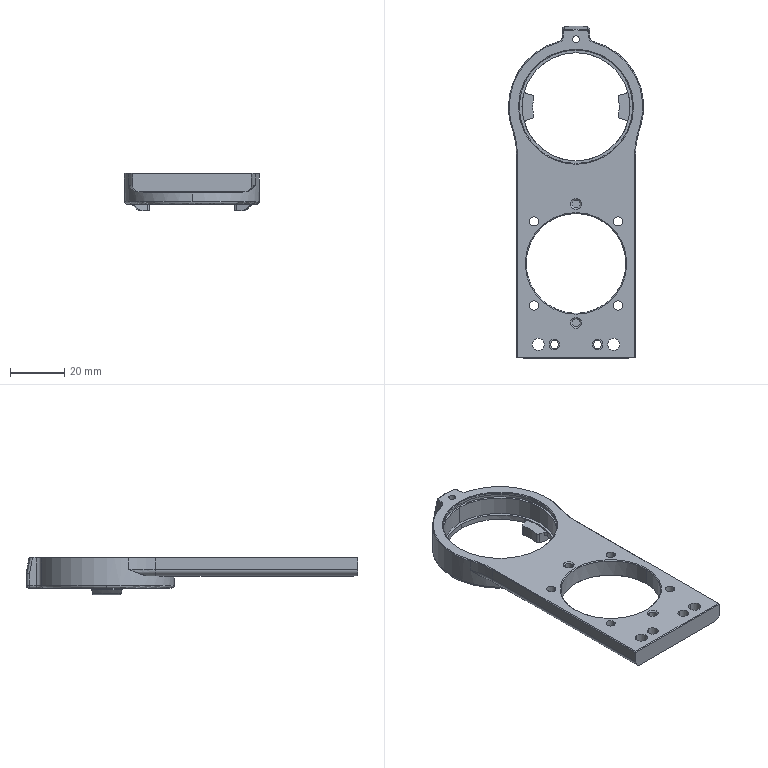NC program | NX | posted with a generic post | part box 50 x 122.9 x 14 mm
Lines 1 to 868 of 10876:
N10 G17 G21 G94 G90
(FLOOR_WALL_COPY , TOOL : D80)
N12 T19 M6
N14 G54
N16 G17 G0 G90 X-45. Y0. S5000 M3
N18 G43 Z30. H19
N20 Z3.8
N22 G94 G1 Z0.8 F1200.
N24 X-40.
N26 X162.9
N28 X167.9
N30 Z3.8
N32 G0 Z30.
N34 X-45.
N36 Z3.1
N38 G1 Z0.1
N40 X-40.
N42 X162.9
N44 X167.9
N46 Z3.1
N48 G0 Z30.
(FLOOR_WALL_COPY_COPY , TOOL : D80)
N50 X-45.
N52 Z3.
N54 G1 Z0.
N56 X-40.
N58 X162.9
N60 X167.9
N62 Z3.
N64 G0 Z30.
N66 M5
(FLOOR_WALL_1 , TOOL : D10)
N68 T15 M6
N70 G54
N72 G17 G0 G90 X28.07 Y0. S9500 M3
N74 G43 Z30. H15
N76 Z1.5
N78 G94 G1 X35.5 Z1.111 F1000.
N80 X19.5 Z0.272
N82 X35.5 Z-0.566
N84 X27.5 Z-0.986
N86 X19.5 F2500.
N88 X35.5
N90 X27.5
N92 Y-4.5
N94 X38.603
N96 G2 X39.534 Y-2.109 R20.
N98 G3 X39.534 Y2.109 R5.
N100 G2 X38.603 Y4.5 R20.
N102 G1 X15.
N104 Y-4.5
N106 X27.5
N108 Y-9.5
N110 X42.704
N112 G2 X44.067 Y-4.218 R15.
N114 G3 X44.067 Y4.218 R10.
N116 G2 X42.704 Y9.5 R15.
N118 G1 X10.
N120 Y-9.5
N122 X27.5
N124 Y-14.5
N126 X48.483
N128 G2 X48.601 Y-6.327 R10.
N130 G3 X48.601 Y6.327 R15.
N132 G2 X48.483 Y14.5 R10.
N134 G1 X5.
N136 Y-14.5
N138 X27.5
N140 Y-19.5
N142 X63.815
N144 G2 X62.867 Y-18. R35.1
N146 G1 X58.872
N148 G2 X54.093 Y-14.469 R5.
N150 G3 X53.581 Y-13.425 R3.7
N152 G2 X53.134 Y-8.435 R5.
N154 G3 X53.134 Y8.435 R20.
N156 G2 X53.581 Y13.425 R5.
N158 G3 X54.093 Y14.469 R3.7
N160 G2 X58.872 Y18. R5.
N162 G1 X62.867
N164 G2 X63.815 Y19.5 R35.1
N166 G1 X0.
N168 Y-19.5
N170 X27.5
N172 Y-24.5
N174 X75.084
N176 G2 X75.476 Y-24.503 R27.5
N178 G1 Y-24.473
N180 G2 X65.852 Y-13. R30.1
N182 G1 X58.872
N184 G3 X57.668 Y-10.544 R8.7
N186 X57.668 Y10.544 R25.
N188 X58.872 Y13. R8.7
N190 G1 X65.852
N192 G2 X75.476 Y24.473 R30.1
N194 G1 Y24.503
N196 G2 X75.084 Y24.5 R27.5
N198 G1 X-5.
N200 Y-24.5
N202 X27.5
N204 Z0.514
N206 G0 X28.07 Y0.
N208 G1 X35.5 Z0.125 F1000.
N210 X19.5 Z-0.714
N212 X35.5 Z-1.552
N214 X27.5 Z-1.971
N216 X19.5 F2500.
N218 X35.5
N220 X27.5
N222 Y-4.5
N224 X38.603
N226 G2 X39.534 Y-2.109 R20.
N228 G3 X39.534 Y2.109 R5.
N230 G2 X38.603 Y4.5 R20.
N232 G1 X15.
N234 Y-4.5
N236 X27.5
N238 Y-9.5
N240 X42.704
N242 G2 X44.067 Y-4.218 R15.
N244 G3 X44.067 Y4.218 R10.
N246 G2 X42.704 Y9.5 R15.
N248 G1 X10.
N250 Y-9.5
N252 X27.5
N254 Y-14.5
N256 X48.483
N258 G2 X48.601 Y-6.327 R10.
N260 G3 X48.601 Y6.327 R15.
N262 G2 X48.483 Y14.5 R10.
N264 G1 X5.
N266 Y-14.5
N268 X27.5
N270 Y-19.5
N272 X63.815
N274 G2 X62.867 Y-18. R35.1
N276 G1 X58.872
N278 G2 X54.093 Y-14.469 R5.
N280 G3 X53.581 Y-13.425 R3.7
N282 G2 X53.134 Y-8.435 R5.
N284 G3 X53.134 Y8.435 R20.
N286 G2 X53.581 Y13.425 R5.
N288 G3 X54.093 Y14.469 R3.7
N290 G2 X58.872 Y18. R5.
N292 G1 X62.867
N294 G2 X63.815 Y19.5 R35.1
N296 G1 X0.
N298 Y-19.5
N300 X27.5
N302 Y-24.5
N304 X75.084
N306 G2 X75.476 Y-24.503 R27.5
N308 G1 Y-24.473
N310 G2 X65.852 Y-13. R30.1
N312 G1 X58.872
N314 G3 X57.668 Y-10.544 R8.7
N316 X57.668 Y10.544 R25.
N318 X58.872 Y13. R8.7
N320 G1 X65.852
N322 G2 X75.476 Y24.473 R30.1
N324 G1 Y24.503
N326 G2 X75.084 Y24.5 R27.5
N328 G1 X-5.
N330 Y-24.5
N332 X27.5
N334 Z-0.471
N336 G0 X28.07 Y0.
N338 G1 X35.5 Z-0.861 F1000.
N340 X19.5 Z-1.699
N342 X35.5 Z-2.538
N344 X27.5 Z-2.957
N346 X19.5 F2500.
N348 X35.5
N350 X27.5
N352 Y-4.5
N354 X38.603
N356 G2 X39.534 Y-2.109 R20.
N358 G3 X39.534 Y2.109 R5.
N360 G2 X38.603 Y4.5 R20.
N362 G1 X15.
N364 Y-4.5
N366 X27.5
N368 Y-9.5
N370 X42.704
N372 G2 X44.067 Y-4.218 R15.
N374 G3 X44.067 Y4.218 R10.
N376 G2 X42.704 Y9.5 R15.
N378 G1 X10.
N380 Y-9.5
N382 X27.5
N384 Y-14.5
N386 X48.483
N388 G2 X48.601 Y-6.327 R10.
N390 G3 X48.601 Y6.327 R15.
N392 G2 X48.483 Y14.5 R10.
N394 G1 X5.
N396 Y-14.5
N398 X27.5
N400 Y-19.5
N402 X63.815
N404 G2 X62.867 Y-18. R35.1
N406 G1 X58.872
N408 G2 X54.093 Y-14.469 R5.
N410 G3 X53.581 Y-13.425 R3.7
N412 G2 X53.134 Y-8.435 R5.
N414 G3 X53.134 Y8.435 R20.
N416 G2 X53.581 Y13.425 R5.
N418 G3 X54.093 Y14.469 R3.7
N420 G2 X58.872 Y18. R5.
N422 G1 X62.867
N424 G2 X63.815 Y19.5 R35.1
N426 G1 X0.
N428 Y-19.5
N430 X27.5
N432 Y-24.5
N434 X75.084
N436 G2 X75.476 Y-24.503 R27.5
N438 G1 Y-24.473
N440 G2 X65.852 Y-13. R30.1
N442 G1 X58.872
N444 G3 X57.668 Y-10.544 R8.7
N446 X57.668 Y10.544 R25.
N448 X58.872 Y13. R8.7
N450 G1 X65.852
N452 G2 X75.476 Y24.473 R30.1
N454 G1 Y24.503
N456 G2 X75.084 Y24.5 R27.5
N458 G1 X-5.
N460 Y-24.5
N462 X27.5
N464 Z-1.457
N466 G0 X28.07 Y0.
N468 G1 X35.5 Z-1.847 F1000.
N470 X19.5 Z-2.685
N472 X35.5 Z-3.524
N474 X27.5 Z-3.943
N476 X19.5 F2500.
N478 X35.5
N480 X27.5
N482 Y-4.5
N484 X38.603
N486 G2 X39.534 Y-2.109 R20.
N488 G3 X39.534 Y2.109 R5.
N490 G2 X38.603 Y4.5 R20.
N492 G1 X15.
N494 Y-4.5
N496 X27.5
N498 Y-9.5
N500 X42.704
N502 G2 X44.067 Y-4.218 R15.
N504 G3 X44.067 Y4.218 R10.
N506 G2 X42.704 Y9.5 R15.
N508 G1 X10.
N510 Y-9.5
N512 X27.5
N514 Y-14.5
N516 X48.483
N518 G2 X48.601 Y-6.327 R10.
N520 G3 X48.601 Y6.327 R15.
N522 G2 X48.483 Y14.5 R10.
N524 G1 X5.
N526 Y-14.5
N528 X27.5
N530 Y-19.5
N532 X63.815
N534 G2 X62.867 Y-18. R35.1
N536 G1 X58.872
N538 G2 X54.093 Y-14.469 R5.
N540 G3 X53.581 Y-13.425 R3.7
N542 G2 X53.134 Y-8.435 R5.
N544 G3 X53.134 Y8.435 R20.
N546 G2 X53.581 Y13.425 R5.
N548 G3 X54.093 Y14.469 R3.7
N550 G2 X58.872 Y18. R5.
N552 G1 X62.867
N554 G2 X63.815 Y19.5 R35.1
N556 G1 X0.
N558 Y-19.5
N560 X27.5
N562 Y-24.5
N564 X75.084
N566 G2 X75.476 Y-24.503 R27.5
N568 G1 Y-24.473
N570 G2 X65.852 Y-13. R30.1
N572 G1 X58.872
N574 G3 X57.668 Y-10.544 R8.7
N576 X57.668 Y10.544 R25.
N578 X58.872 Y13. R8.7
N580 G1 X65.852
N582 G2 X75.476 Y24.473 R30.1
N584 G1 Y24.503
N586 G2 X75.084 Y24.5 R27.5
N588 G1 X-5.
N590 Y-24.5
N592 X27.5
N594 Z-2.443
N596 G0 X28.07 Y0.
N598 G1 X35.5 Z-2.832 F1000.
N600 X19.5 Z-3.671
N602 X35.5 Z-4.509
N604 X27.5 Z-4.929
N606 X19.5 F2500.
N608 X35.5
N610 X27.5
N612 Y-4.5
N614 X38.603
N616 G2 X39.534 Y-2.109 R20.
N618 G3 X39.534 Y2.109 R5.
N620 G2 X38.603 Y4.5 R20.
N622 G1 X15.
N624 Y-4.5
N626 X27.5
N628 Y-9.5
N630 X42.704
N632 G2 X44.067 Y-4.218 R15.
N634 G3 X44.067 Y4.218 R10.
N636 G2 X42.704 Y9.5 R15.
N638 G1 X10.
N640 Y-9.5
N642 X27.5
N644 Y-14.5
N646 X48.483
N648 G2 X48.601 Y-6.327 R10.
N650 G3 X48.601 Y6.327 R15.
N652 G2 X48.483 Y14.5 R10.
N654 G1 X5.
N656 Y-14.5
N658 X27.5
N660 Y-19.5
N662 X63.815
N664 G2 X62.867 Y-18. R35.1
N666 G1 X58.872
N668 G2 X54.093 Y-14.469 R5.
N670 G3 X53.581 Y-13.425 R3.7
N672 G2 X53.134 Y-8.435 R5.
N674 G3 X53.134 Y8.435 R20.
N676 G2 X53.581 Y13.425 R5.
N678 G3 X54.093 Y14.469 R3.7
N680 G2 X58.872 Y18. R5.
N682 G1 X62.867
N684 G2 X63.815 Y19.5 R35.1
N686 G1 X0.
N688 Y-19.5
N690 X27.5
N692 Y-24.5
N694 X75.084
N696 G2 X75.476 Y-24.503 R27.5
N698 G1 Y-24.473
N700 G2 X65.852 Y-13. R30.1
N702 G1 X58.872
N704 G3 X57.668 Y-10.544 R8.7
N706 X57.668 Y10.544 R25.
N708 X58.872 Y13. R8.7
N710 G1 X65.852
N712 G2 X75.476 Y24.473 R30.1
N714 G1 Y24.503
N716 G2 X75.084 Y24.5 R27.5
N718 G1 X-5.
N720 Y-24.5
N722 X27.5
N724 Z-3.429
N726 G0 X28.07 Y0.
N728 G1 X35.5 Z-3.818 F1000.
N730 X19.5 Z-4.656
N732 X35.5 Z-5.495
N734 X27.5 Z-5.914
N736 X19.5 F2500.
N738 X35.5
N740 X27.5
N742 Y-4.5
N744 X38.603
N746 G2 X39.534 Y-2.109 R20.
N748 G3 X39.534 Y2.109 R5.
N750 G2 X38.603 Y4.5 R20.
N752 G1 X15.
N754 Y-4.5
N756 X27.5
N758 Y-9.5
N760 X42.704
N762 G2 X44.067 Y-4.218 R15.
N764 G3 X44.067 Y4.218 R10.
N766 G2 X42.704 Y9.5 R15.
N768 G1 X10.
N770 Y-9.5
N772 X27.5
N774 Y-14.5
N776 X48.483
N778 G2 X48.601 Y-6.327 R10.
N780 G3 X48.601 Y6.327 R15.
N782 G2 X48.483 Y14.5 R10.
N784 G1 X5.
N786 Y-14.5
N788 X27.5
N790 Y-19.5
N792 X63.815
N794 G2 X62.867 Y-18. R35.1
N796 G1 X58.872
N798 G2 X54.093 Y-14.469 R5.
N800 G3 X53.581 Y-13.425 R3.7
N802 G2 X53.134 Y-8.435 R5.
N804 G3 X53.134 Y8.435 R20.
N806 G2 X53.581 Y13.425 R5.
N808 G3 X54.093 Y14.469 R3.7
N810 G2 X58.872 Y18. R5.
N812 G1 X62.867
N814 G2 X63.815 Y19.5 R35.1
N816 G1 X0.
N818 Y-19.5
N820 X27.5
N822 Y-24.5
N824 X75.084
N826 G2 X75.476 Y-24.503 R27.5
N828 G1 Y-24.473
N830 G2 X65.852 Y-13. R30.1
N832 G1 X58.872
N834 G3 X57.668 Y-10.544 R8.7
N836 X57.668 Y10.544 R25.
N838 X58.872 Y13. R8.7
N840 G1 X65.852
N842 G2 X75.476 Y24.473 R30.1
N844 G1 Y24.503
N846 G2 X75.084 Y24.5 R27.5
N848 G1 X-5.
N850 Y-24.5
N852 X27.5
N854 Z-4.414
N856 G0 X28.07 Y0.
N858 G1 X35.5 Z-4.804 F1000.
N860 X19.5 Z-5.642
N862 X35.5 Z-6.481
N864 X27.5 Z-6.9
N866 X19.5 F2500.
N868 X35.5
N870 X27.5
N872 Y-4.5
N874 X38.603
N876 G2 X39.534 Y-2.109 R20.
N878 G3 X39.534 Y2.109 R5.
N880 G2 X38.603 Y4.5 R20.
N882 G1 X15.
N884 Y-4.5
N886 X27.5
N888 Y-9.5
N890 X42.704
N892 G2 X44.067 Y-4.218 R15.
N894 G3 X44.067 Y4.218 R10.
N896 G2 X42.704 Y9.5 R15.
N898 G1 X10.
N900 Y-9.5
N902 X27.5
N904 Y-14.5
N906 X48.483
N908 G2 X48.601 Y-6.327 R10.
N910 G3 X48.601 Y6.327 R15.
N912 G2 X48.483 Y14.5 R10.
N914 G1 X5.
N916 Y-14.5
N918 X27.5
N920 Y-19.5
N922 X63.815
N924 G2 X62.867 Y-18. R35.1
N926 G1 X58.872
N928 G2 X54.093 Y-14.469 R5.
N930 G3 X53.581 Y-13.425 R3.7
N932 G2 X53.134 Y-8.435 R5.
N934 G3 X53.134 Y8.435 R20.
N936 G2 X53.581 Y13.425 R5.
N938 G3 X54.093 Y14.469 R3.7
N940 G2 X58.872 Y18. R5.
N942 G1 X62.867
N944 G2 X63.815 Y19.5 R35.1
N946 G1 X0.
N948 Y-19.5
N950 X27.5
N952 Y-24.5
N954 X75.084
N956 G2 X75.476 Y-24.503 R27.5
N958 G1 Y-24.473
N960 G2 X65.852 Y-13. R30.1
N962 G1 X58.872
N964 G3 X57.668 Y-10.544 R8.7
N966 X57.668 Y10.544 R25.
N968 X58.872 Y13. R8.7
N970 G1 X65.852
N972 G2 X75.476 Y24.473 R30.1
N974 G1 Y24.503
N976 G2 X75.084 Y24.5 R27.5
N978 G1 X-5.
N980 Y-24.5
N982 X27.5
N984 Z-5.4
N986 G0 Z30.
(FLOOR_WALL_1_COPY , TOOL : D10)
N988 X102.876 Y-13.629
N990 Z1.5
N992 G1 X103.115 Y-14.182 Z1.468 F1000.
N994 X104.9 Y-20.842 Z1.107
N996 X105.942 Y-20.247 Z1.044
N998 X108.408 Y-18.44 Z0.884
N1000 X110.624 Y-16.335 Z0.724
N1002 X112.556 Y-13.965 Z0.564
N1004 X114.17 Y-11.369 Z0.403
N1006 X115.442 Y-8.589 Z0.243
N1008 X115.985 Y-6.927 Z0.151
N1010 X116.364 Y-6.238 Z0.11
N1012 X116.846 Y-5.617 Z0.069
N1014 X117.668 Y-4.89 Z0.012
N1016 X118.787 Y-4.296 Z-0.055
N1018 X120.02 Y-4. Z-0.121
N1020 X120.568 Z-0.15
N1022 X121.622 Z-0.205
N1024 X121.804 Y-2.695 Z-0.274
N1026 X121.93 Y0. Z-0.416
N1028 X121.804 Y2.696 Z-0.557
N1030 X121.622 Y4. Z-0.626
N1032 X120.02 Z-0.71
N1034 X118.882 Y4.261 Z-0.771
N1036 X118.389 Y4.5 Z-0.8
N1038 X116.209 Y0.
N1040 G2 X113.946 Y1.507 R10. F2500.
N1042 X113.946 Y-1.507 R21.
N1044 X116.209 Y0. R10.
N1046 G1 X117.879 Y4.784
N1048 G2 X115.815 Y7.448 R5.
N1050 G3 X104.9 Y20.842 R24.
N1052 G1 X103.284 Y14.814
N1054 G2 X102.458 Y12.905 R7.1
N1056 X102.458 Y-12.905 R16.
N1058 X103.284 Y-14.814 R7.1
N1060 G1 X104.9 Y-20.842
N1062 X103.934 Y-21.101
N1064 X104.94 Y-24.857
N1066 X100.014 Y-26.177
N1068 G2 X85.986 Y-26.177 R27.1
N1070 G1 X81.06 Y-24.857
N1072 X83.681 Y-15.072
N1074 G2 X85.217 Y-12.381 R6.1
N1076 G1 X84.554 Y-12.203
N1078 X84.51 Y-12.366
N1080 G2 X84.51 Y12.366 R15.
N1082 G1 X84.554 Y12.203
N1084 X85.217 Y12.381
N1086 G2 X83.681 Y15.072 R6.1
N1088 G1 X81.06 Y24.857
N1090 X85.986 Y26.177
N1092 G2 X100.014 Y26.177 R27.1
N1094 G1 X104.94 Y24.857
N1096 X102.319 Y15.072
N1098 G2 X100.783 Y12.381 R6.1
N1100 G1 X101.446 Y12.203
N1102 X101.49 Y12.366
N1104 G2 X101.49 Y-12.366 R15.
N1106 G1 X101.446 Y-12.203
N1108 X100.783 Y-12.381
N1110 G2 X102.319 Y-15.072 R6.1
N1112 G1 X103.934 Y-21.101
N1114 X104.9 Y-20.842
N1116 G3 X115.815 Y-7.448 R24.
N1118 G2 X120.568 Y-4. R5.
N1120 G1 X121.622
N1122 G3 X121.622 Y4. R28.9
N1124 G1 X120.568
N1126 G2 X117.879 Y4.784 R5.
N1128 G1 X120.568 Y9.
N1130 G3 X78.621 Y25.184 R29.
N1132 G1 X81.1 Y20.842
N1134 G3 X81.1 Y-20.842 R24.
N1136 G1 X82.716 Y-14.814
N1138 G2 X83.542 Y-12.905 R7.1
N1140 X83.542 Y12.905 R16.
N1142 X82.716 Y14.814 R7.1
N1144 G1 X81.1 Y20.842
N1146 X78.621 Y25.184
N1148 G3 X120.568 Y-9. R-29.
N1150 G1 X125.972
N1152 X126.574 Y-4.692
N1154 G3 X126.574 Y4.692 R33.9
N1156 G1 X125.972 Y9.
N1158 X120.568
N1160 Z0.7
N1162 G0 X102.876 Y-13.629
N1164 G1 X103.115 Y-14.182 Z0.668 F1000.
N1166 X104.9 Y-20.842 Z0.307
N1168 X105.942 Y-20.247 Z0.244
N1170 X108.408 Y-18.44 Z0.084
N1172 X110.624 Y-16.335 Z-0.076
N1174 X112.556 Y-13.965 Z-0.236
N1176 X114.17 Y-11.369 Z-0.397
N1178 X115.442 Y-8.589 Z-0.557
N1180 X115.985 Y-6.927 Z-0.649
N1182 X116.364 Y-6.238 Z-0.69
N1184 X116.846 Y-5.617 Z-0.731
N1186 X117.668 Y-4.89 Z-0.788
N1188 X118.787 Y-4.296 Z-0.855
N1190 X120.02 Y-4. Z-0.921
N1192 X120.568 Z-0.95
N1194 X121.622 Z-1.005
N1196 X121.804 Y-2.695 Z-1.074
N1198 X121.93 Y0. Z-1.216
N1200 X121.804 Y2.696 Z-1.357
N1202 X121.622 Y4. Z-1.426
N1204 X120.02 Z-1.51
N1206 X118.882 Y4.261 Z-1.571
N1208 X118.389 Y4.5 Z-1.6
N1210 X116.209 Y0.
N1212 G2 X113.946 Y1.507 R10. F2500.
N1214 X113.946 Y-1.507 R21.
N1216 X116.209 Y0. R10.
N1218 G1 X117.879 Y4.784
N1220 G2 X115.815 Y7.448 R5.
N1222 G3 X104.9 Y20.842 R24.
N1224 G1 X103.284 Y14.814
N1226 G2 X102.458 Y12.905 R7.1
N1228 X102.458 Y-12.905 R16.
N1230 X103.284 Y-14.814 R7.1
N1232 G1 X104.9 Y-20.842
N1234 X103.934 Y-21.101
N1236 X104.94 Y-24.857
N1238 X100.014 Y-26.177
N1240 G2 X85.986 Y-26.177 R27.1
N1242 G1 X81.06 Y-24.857
N1244 X83.681 Y-15.072
N1246 G2 X85.217 Y-12.381 R6.1
N1248 G1 X84.554 Y-12.203
N1250 X84.51 Y-12.366
N1252 G2 X84.51 Y12.366 R15.
N1254 G1 X84.554 Y12.203
N1256 X85.217 Y12.381
N1258 G2 X83.681 Y15.072 R6.1
N1260 G1 X81.06 Y24.857
N1262 X85.986 Y26.177
N1264 G2 X100.014 Y26.177 R27.1
N1266 G1 X104.94 Y24.857
N1268 X102.319 Y15.072
N1270 G2 X100.783 Y12.381 R6.1
N1272 G1 X101.446 Y12.203
N1274 X101.49 Y12.366
N1276 G2 X101.49 Y-12.366 R15.
N1278 G1 X101.446 Y-12.203
N1280 X100.783 Y-12.381
N1282 G2 X102.319 Y-15.072 R6.1
N1284 G1 X103.934 Y-21.101
N1286 X104.9 Y-20.842
N1288 G3 X115.815 Y-7.448 R24.
N1290 G2 X120.568 Y-4. R5.
N1292 G1 X121.622
N1294 G3 X121.622 Y4. R28.9
N1296 G1 X120.568
N1298 G2 X117.879 Y4.784 R5.
N1300 G1 X120.568 Y9.
N1302 G3 X78.621 Y25.184 R29.
N1304 G1 X81.1 Y20.842
N1306 G3 X81.1 Y-20.842 R24.
N1308 G1 X82.716 Y-14.814
N1310 G2 X83.542 Y-12.905 R7.1
N1312 X83.542 Y12.905 R16.
N1314 X82.716 Y14.814 R7.1
N1316 G1 X81.1 Y20.842
N1318 X78.621 Y25.184
N1320 G3 X120.568 Y-9. R-29.
N1322 G1 X125.972
N1324 X126.574 Y-4.692
N1326 G3 X126.574 Y4.692 R33.9
N1328 G1 X125.972 Y9.
N1330 X120.568
N1332 Z-0.1
N1334 G0 X102.876 Y-13.629
N1336 G1 X103.115 Y-14.182 Z-0.132 F1000.
N1338 X104.9 Y-20.842 Z-0.493
N1340 X105.942 Y-20.247 Z-0.556
N1342 X108.408 Y-18.44 Z-0.716
N1344 X110.624 Y-16.335 Z-0.876
N1346 X112.556 Y-13.965 Z-1.036
N1348 X114.17 Y-11.369 Z-1.197
N1350 X115.442 Y-8.589 Z-1.357
N1352 X115.985 Y-6.927 Z-1.449
N1354 X116.364 Y-6.238 Z-1.49
N1356 X116.846 Y-5.617 Z-1.531
N1358 X117.668 Y-4.89 Z-1.588
N1360 X118.787 Y-4.296 Z-1.655
N1362 X120.02 Y-4. Z-1.721
N1364 X120.568 Z-1.75
N1366 X121.622 Z-1.805
N1368 X121.804 Y-2.695 Z-1.874
N1370 X121.93 Y0. Z-2.016
N1372 X121.804 Y2.696 Z-2.157
N1374 X121.622 Y4. Z-2.226
N1376 X120.02 Z-2.31
N1378 X118.882 Y4.261 Z-2.371
N1380 X118.389 Y4.5 Z-2.4
N1382 X116.209 Y0.
N1384 G2 X113.946 Y1.507 R10. F2500.
N1386 X113.946 Y-1.507 R21.
N1388 X116.209 Y0. R10.
N1390 G1 X117.879 Y4.784
N1392 G2 X115.815 Y7.448 R5.
N1394 G3 X104.9 Y20.842 R24.
N1396 G1 X103.284 Y14.814
N1398 G2 X102.458 Y12.905 R7.1
N1400 X102.458 Y-12.905 R16.
N1402 X103.284 Y-14.814 R7.1
N1404 G1 X104.9 Y-20.842
N1406 X103.934 Y-21.101
N1408 X104.94 Y-24.857
N1410 X100.014 Y-26.177
N1412 G2 X85.986 Y-26.177 R27.1
N1414 G1 X81.06 Y-24.857
N1416 X83.681 Y-15.072
N1418 G2 X85.217 Y-12.381 R6.1
N1420 G1 X84.554 Y-12.203
N1422 X84.51 Y-12.366
N1424 G2 X84.51 Y12.366 R15.
N1426 G1 X84.554 Y12.203
N1428 X85.217 Y12.381
N1430 G2 X83.681 Y15.072 R6.1
N1432 G1 X81.06 Y24.857
N1434 X85.986 Y26.177
N1436 G2 X100.014 Y26.177 R27.1
N1438 G1 X104.94 Y24.857
N1440 X102.319 Y15.072
N1442 G2 X100.783 Y12.381 R6.1
N1444 G1 X101.446 Y12.203
N1446 X101.49 Y12.366
N1448 G2 X101.49 Y-12.366 R15.
N1450 G1 X101.446 Y-12.203
N1452 X100.783 Y-12.381
N1454 G2 X102.319 Y-15.072 R6.1
N1456 G1 X103.934 Y-21.101
N1458 X104.9 Y-20.842
N1460 G3 X115.815 Y-7.448 R24.
N1462 G2 X120.568 Y-4. R5.
N1464 G1 X121.622
N1466 G3 X121.622 Y4. R28.9
N1468 G1 X120.568
N1470 G2 X117.879 Y4.784 R5.
N1472 G1 X120.568 Y9.
N1474 G3 X78.621 Y25.184 R29.
N1476 G1 X81.1 Y20.842
N1478 G3 X81.1 Y-20.842 R24.
N1480 G1 X82.716 Y-14.814
N1482 G2 X83.542 Y-12.905 R7.1
N1484 X83.542 Y12.905 R16.
N1486 X82.716 Y14.814 R7.1
N1488 G1 X81.1 Y20.842
N1490 X78.621 Y25.184
N1492 G3 X120.568 Y-9. R-29.
N1494 G1 X125.972
N1496 X126.574 Y-4.692
N1498 G3 X126.574 Y4.692 R33.9
N1500 G1 X125.972 Y9.
N1502 X120.568
N1504 Z-0.9
N1506 G0 Z30.
(ZLEVEL_PROFILE_COPY_2 , TOOL : D10)
N1508 X80.595 Y-19.987
N1510 Z0.105
N1512 G1 Z-0.895 F1000.
N1514 X82.055 Y-19.596
N1516 G3 X82.762 Y-18.889 R1.
N1518 G1 X83.778 Y-15.098 F2000.
N1520 G2 X90.783 Y-10.774 R6.
N1522 G3 X95.217 Y-10.774 R11.
N1524 G2 X102.222 Y-15.098 R6.
N1526 G1 X103.238 Y-18.889
N1528 G3 X103.945 Y-19.596 R1.
N1530 G1 X105.405 Y-19.987
N1532 Z0.105
N1534 G0 Z30.
N1536 X80.363 Y-20.852
N1538 Z-0.79
N1540 G1 Z-1.79 F1000.
N1542 X81.824 Y-20.461
N1544 G3 X82.531 Y-19.753 R1.
N1546 G1 X83.778 Y-15.098 F2000.
N1548 G2 X90.783 Y-10.774 R6.
N1550 G3 X95.217 Y-10.774 R11.
N1552 G2 X102.222 Y-15.098 R6.
N1554 G1 X103.469 Y-19.753
N1556 G3 X104.176 Y-20.461 R1.
N1558 G1 X105.637 Y-20.852
N1560 Z-0.79
N1562 G0 Z30.
N1564 X105.405 Y19.987
N1566 Z0.105
N1568 G1 Z-0.895 F1000.
N1570 X103.945 Y19.596
N1572 G3 X103.238 Y18.889 R1.
N1574 G1 X102.222 Y15.098 F2000.
N1576 G2 X95.217 Y10.774 R6.
N1578 G3 X90.783 Y10.774 R11.
N1580 G2 X83.778 Y15.098 R6.
N1582 G1 X82.762 Y18.889
N1584 G3 X82.055 Y19.596 R1.
N1586 G1 X80.595 Y19.987
N1588 Z0.105
N1590 G0 Z30.
N1592 X105.637 Y20.852
N1594 Z-0.79
N1596 G1 Z-1.79 F1000.
N1598 X104.176 Y20.461
N1600 G3 X103.469 Y19.753 R1.
N1602 G1 X102.222 Y15.098 F2000.
N1604 G2 X95.217 Y10.774 R6.
N1606 G3 X90.783 Y10.774 R11.
N1608 G2 X83.778 Y15.098 R6.
N1610 G1 X82.531 Y19.753
N1612 G3 X81.824 Y20.461 R1.
N1614 G1 X80.363 Y20.852
N1616 Z-0.79
N1618 G0 X89.551 Y-8.651 Z-1.685
N1620 G1 Z-2.685 F1000.
N1622 X90.035 Y-10.11
N1624 G3 X90.783 Y-10.774 R1.
N1626 X95.217 Y-10.774 R11. F2000.
N1628 G2 X100.956 Y-12.716 R6.
N1630 G3 X100.956 Y12.716 R15.
N1632 G2 X95.217 Y10.774 R6.
N1634 G3 X90.783 Y10.774 R11.
N1636 G2 X85.044 Y12.716 R6.
N1638 G3 X85.044 Y-12.716 R15.
N1640 G2 X90.783 Y-10.774 R6.
N1642 G3 X91.732 Y-10.459 R1.
N1644 G1 X93.029 Y-9.
N1646 Z-1.685
N1648 G0 X89.551 Y-8.651 Z-2.58
N1650 G1 Z-3.58 F1000.
N1652 X90.035 Y-10.11
N1654 G3 X90.783 Y-10.774 R1.
N1656 X95.217 Y-10.774 R11. F2000.
N1658 G2 X100.956 Y-12.716 R6.
N1660 G3 X100.956 Y12.716 R15.
N1662 G2 X95.217 Y10.774 R6.
N1664 G3 X90.783 Y10.774 R11.
N1666 G2 X85.044 Y12.716 R6.
N1668 G3 X85.044 Y-12.716 R15.
N1670 G2 X90.783 Y-10.774 R6.
N1672 G3 X91.732 Y-10.459 R1.
N1674 G1 X93.029 Y-9.
N1676 Z-2.58
N1678 G0 X89.551 Y-8.651 Z-3.475
N1680 G1 Z-4.475 F1000.
N1682 X90.035 Y-10.11
N1684 G3 X90.783 Y-10.774 R1.
N1686 X95.217 Y-10.774 R11. F2000.
N1688 G2 X100.956 Y-12.716 R6.
N1690 G3 X100.956 Y12.716 R15.
N1692 G2 X95.217 Y10.774 R6.
N1694 G3 X90.783 Y10.774 R11.
N1696 G2 X85.044 Y12.716 R6.
N1698 G3 X85.044 Y-12.716 R15.
N1700 G2 X90.783 Y-10.774 R6.
N1702 G3 X91.732 Y-10.459 R1.
N1704 G1 X93.029 Y-9.
N1706 Z-3.475
N1708 G0 Z30.
N1710 M5